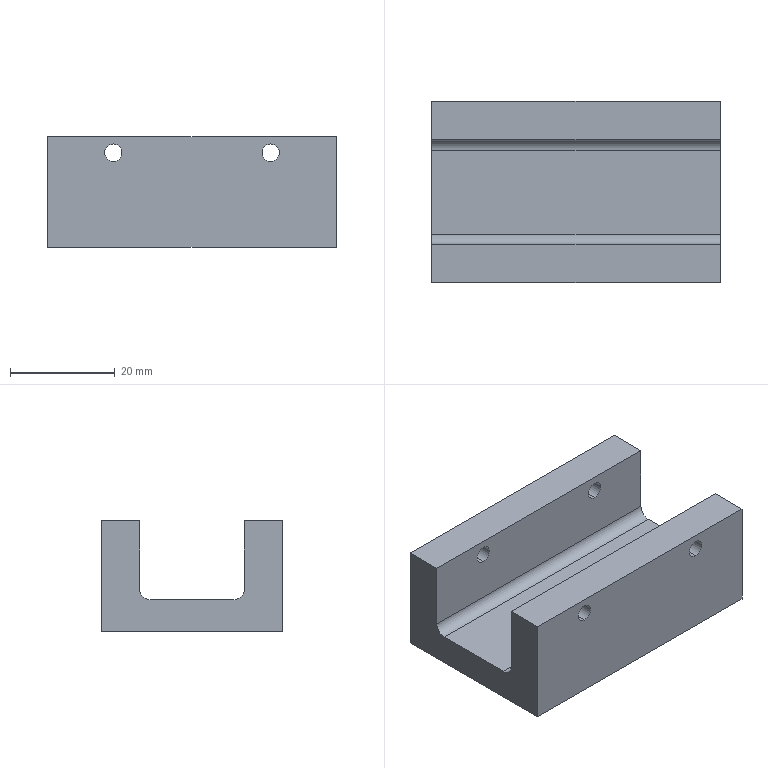Part | STEP file | GLSJ-10-15_default | 1 solid | 36 faces | box 55 x 34.5 x 21 mm | volume 22837 mm3 | cylinder 18 | plane 10 | cone 8 | commonest cylinder face diameters 3.3 x16 4 x2